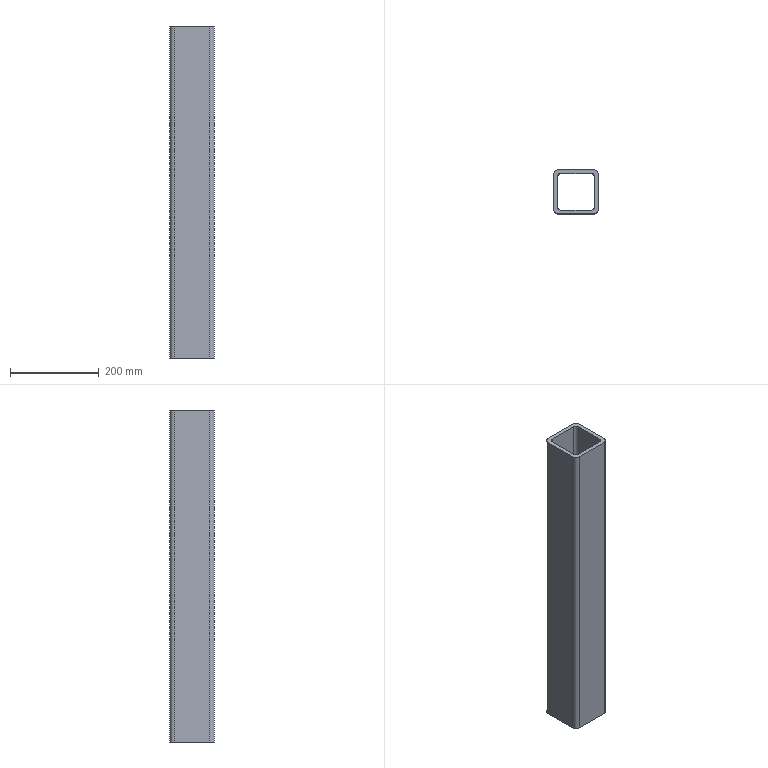Part | SolidWorks | features BaseBody 1 | 1 solid | 18 faces | box 100 x 100 x 750 mm | volume 2184823 mm3 | plane 10 | cylinder 8 | commonest cylinder face diameters 16 x4 20 x4
STEP:
#1=CARTESIAN_POINT('',(90.,-3.65,750.));
#2=VERTEX_POINT('',#1);
#3=CARTESIAN_POINT('',(90.,-3.65,0.));
#4=VERTEX_POINT('',#3);
#5=CARTESIAN_POINT('',(90.,-3.65,750.));
#6=DIRECTION('',(0.,0.,-1.));
#7=VECTOR('',#6,1000.);
#8=LINE('',#5,#7);
#9=EDGE_CURVE('',#2,#4,#8,.T.);
#10=ORIENTED_EDGE('',*,*,#9,.F.);
#11=CARTESIAN_POINT('',(10.,-3.65,750.));
#12=VERTEX_POINT('',#11);
#13=CARTESIAN_POINT('',(10.,-3.65,750.));
#14=DIRECTION('',(1.,0.,0.));
#15=VECTOR('',#14,1000.);
#16=LINE('',#13,#15);
#17=EDGE_CURVE('',#12,#2,#16,.T.);
#18=ORIENTED_EDGE('',*,*,#17,.F.);
#19=CARTESIAN_POINT('',(10.,-3.65,0.));
#20=VERTEX_POINT('',#19);
#21=CARTESIAN_POINT('',(10.,-3.65,750.));
#22=DIRECTION('',(0.,0.,1.));
#23=VECTOR('',#22,1000.);
#24=LINE('',#21,#23);
#25=EDGE_CURVE('',#20,#12,#24,.T.);
#26=ORIENTED_EDGE('',*,*,#25,.F.);
#27=CARTESIAN_POINT('',(10.,-3.65,0.));
#28=DIRECTION('',(-1.,0.,0.));
#29=VECTOR('',#28,1000.);
#30=LINE('',#27,#29);
#31=EDGE_CURVE('',#4,#20,#30,.T.);
#32=ORIENTED_EDGE('',*,*,#31,.F.);
#33=EDGE_LOOP('',(#10,#18,#26,#32));
#34=FACE_OUTER_BOUND('',#33,.T.);
#35=CARTESIAN_POINT('',(10.,-3.65,750.));
#36=DIRECTION('',(0.,1.,0.));
#37=DIRECTION('',(-1.,0.,0.));
#38=AXIS2_PLACEMENT_3D('',#35,#36,#37);
#39=PLANE('',#38);
#40=ADVANCED_FACE('',(#34),#39,.F.);
#41=CARTESIAN_POINT('',(84.,4.35,0.));
#42=VERTEX_POINT('',#41);
#43=CARTESIAN_POINT('',(16.,4.35,0.));
#44=VERTEX_POINT('',#43);
#45=CARTESIAN_POINT('',(10.,4.35,0.));
#46=DIRECTION('',(-1.,0.,0.));
#47=VECTOR('',#46,1000.);
#48=LINE('',#45,#47);
#49=EDGE_CURVE('',#42,#44,#48,.T.);
#50=ORIENTED_EDGE('',*,*,#49,.F.);
#51=CARTESIAN_POINT('',(92.,12.35,0.));
#52=VERTEX_POINT('',#51);
#53=CARTESIAN_POINT('',(84.,12.35,0.));
#54=DIRECTION('',(0.,0.,-1.));
#55=DIRECTION('',(-1.,0.,0.));
#56=AXIS2_PLACEMENT_3D('',#53,#54,#55);
#57=CIRCLE('',#56,8.);
#58=EDGE_CURVE('',#52,#42,#57,.T.);
#59=ORIENTED_EDGE('',*,*,#58,.F.);
#60=CARTESIAN_POINT('',(92.,80.35,0.));
#61=VERTEX_POINT('',#60);
#62=CARTESIAN_POINT('',(92.,6.35,0.));
#63=DIRECTION('',(0.,-1.,0.));
#64=VECTOR('',#63,1000.);
#65=LINE('',#62,#64);
#66=EDGE_CURVE('',#61,#52,#65,.T.);
#67=ORIENTED_EDGE('',*,*,#66,.F.);
#68=CARTESIAN_POINT('',(84.,88.35,0.));
#69=VERTEX_POINT('',#68);
#70=CARTESIAN_POINT('',(84.,80.35,0.));
#71=DIRECTION('',(0.,0.,-1.));
#72=DIRECTION('',(-1.,0.,0.));
#73=AXIS2_PLACEMENT_3D('',#70,#71,#72);
#74=CIRCLE('',#73,8.);
#75=EDGE_CURVE('',#69,#61,#74,.T.);
#76=ORIENTED_EDGE('',*,*,#75,.F.);
#77=CARTESIAN_POINT('',(16.,88.35,0.));
#78=VERTEX_POINT('',#77);
#79=CARTESIAN_POINT('',(10.,88.35,0.));
#80=DIRECTION('',(1.,0.,0.));
#81=VECTOR('',#80,1000.);
#82=LINE('',#79,#81);
#83=EDGE_CURVE('',#78,#69,#82,.T.);
#84=ORIENTED_EDGE('',*,*,#83,.F.);
#85=CARTESIAN_POINT('',(8.,80.35,0.));
#86=VERTEX_POINT('',#85);
#87=CARTESIAN_POINT('',(16.,80.35,0.));
#88=DIRECTION('',(0.,0.,-1.));
#89=DIRECTION('',(-1.,0.,0.));
#90=AXIS2_PLACEMENT_3D('',#87,#88,#89);
#91=CIRCLE('',#90,8.);
#92=EDGE_CURVE('',#86,#78,#91,.T.);
#93=ORIENTED_EDGE('',*,*,#92,.F.);
#94=CARTESIAN_POINT('',(8.,12.35,0.));
#95=VERTEX_POINT('',#94);
#96=CARTESIAN_POINT('',(8.,6.35,0.));
#97=DIRECTION('',(0.,1.,0.));
#98=VECTOR('',#97,1000.);
#99=LINE('',#96,#98);
#100=EDGE_CURVE('',#95,#86,#99,.T.);
#101=ORIENTED_EDGE('',*,*,#100,.F.);
#102=CARTESIAN_POINT('',(16.,12.35,0.));
#103=DIRECTION('',(0.,0.,-1.));
#104=DIRECTION('',(-1.,0.,0.));
#105=AXIS2_PLACEMENT_3D('',#102,#103,#104);
#106=CIRCLE('',#105,8.);
#107=EDGE_CURVE('',#44,#95,#106,.T.);
#108=ORIENTED_EDGE('',*,*,#107,.F.);
#109=EDGE_LOOP('',(#50,#59,#67,#76,#84,#93,#101,#108));
#110=FACE_BOUND('',#109,.T.);
#111=CARTESIAN_POINT('',(0.,86.35,0.));
#112=VERTEX_POINT('',#111);
#113=CARTESIAN_POINT('',(0.,6.35,0.));
#114=VERTEX_POINT('',#113);
#115=CARTESIAN_POINT('',(0.,6.35,0.));
#116=DIRECTION('',(0.,-1.,0.));
#117=VECTOR('',#116,1000.);
#118=LINE('',#115,#117);
#119=EDGE_CURVE('',#112,#114,#118,.T.);
#120=ORIENTED_EDGE('',*,*,#119,.F.);
#121=CARTESIAN_POINT('',(10.,96.35,0.));
#122=VERTEX_POINT('',#121);
#123=CARTESIAN_POINT('',(10.,86.35,0.));
#124=DIRECTION('',(0.,0.,1.));
#125=DIRECTION('',(-1.,0.,0.));
#126=AXIS2_PLACEMENT_3D('',#123,#124,#125);
#127=CIRCLE('',#126,10.);
#128=EDGE_CURVE('',#122,#112,#127,.T.);
#129=ORIENTED_EDGE('',*,*,#128,.F.);
#130=CARTESIAN_POINT('',(90.,96.35,0.));
#131=VERTEX_POINT('',#130);
#132=CARTESIAN_POINT('',(10.,96.35,0.));
#133=DIRECTION('',(-1.,0.,0.));
#134=VECTOR('',#133,1000.);
#135=LINE('',#132,#134);
#136=EDGE_CURVE('',#131,#122,#135,.T.);
#137=ORIENTED_EDGE('',*,*,#136,.F.);
#138=CARTESIAN_POINT('',(100.,86.35,0.));
#139=VERTEX_POINT('',#138);
#140=CARTESIAN_POINT('',(90.,86.35,0.));
#141=DIRECTION('',(0.,0.,1.));
#142=DIRECTION('',(-1.,0.,0.));
#143=AXIS2_PLACEMENT_3D('',#140,#141,#142);
#144=CIRCLE('',#143,10.);
#145=EDGE_CURVE('',#139,#131,#144,.T.);
#146=ORIENTED_EDGE('',*,*,#145,.F.);
#147=CARTESIAN_POINT('',(100.,6.35,0.));
#148=VERTEX_POINT('',#147);
#149=CARTESIAN_POINT('',(100.,6.35,0.));
#150=DIRECTION('',(0.,1.,0.));
#151=VECTOR('',#150,1000.);
#152=LINE('',#149,#151);
#153=EDGE_CURVE('',#148,#139,#152,.T.);
#154=ORIENTED_EDGE('',*,*,#153,.F.);
#155=CARTESIAN_POINT('',(90.,6.35,0.));
#156=DIRECTION('',(0.,0.,1.));
#157=DIRECTION('',(-1.,0.,0.));
#158=AXIS2_PLACEMENT_3D('',#155,#156,#157);
#159=CIRCLE('',#158,10.);
#160=EDGE_CURVE('',#4,#148,#159,.T.);
#161=ORIENTED_EDGE('',*,*,#160,.F.);
#162=ORIENTED_EDGE('',*,*,#31,.T.);
#163=CARTESIAN_POINT('',(10.,6.35,0.));
#164=DIRECTION('',(0.,0.,1.));
#165=DIRECTION('',(-1.,0.,0.));
#166=AXIS2_PLACEMENT_3D('',#163,#164,#165);
#167=CIRCLE('',#166,10.);
#168=EDGE_CURVE('',#114,#20,#167,.T.);
#169=ORIENTED_EDGE('',*,*,#168,.F.);
#170=EDGE_LOOP('',(#120,#129,#137,#146,#154,#161,#162,#169));
#171=FACE_OUTER_BOUND('',#170,.T.);
#172=CARTESIAN_POINT('',(10.,6.35,0.));
#173=DIRECTION('',(0.,0.,1.));
#174=DIRECTION('',(1.,0.,0.));
#175=AXIS2_PLACEMENT_3D('',#172,#173,#174);
#176=PLANE('',#175);
#177=ADVANCED_FACE('',(#110,#171),#176,.F.);
#178=CARTESIAN_POINT('',(100.,6.35,750.));
#179=VERTEX_POINT('',#178);
#180=CARTESIAN_POINT('',(90.,6.35,750.));
#181=DIRECTION('',(0.,0.,-1.));
#182=DIRECTION('',(-1.,0.,0.));
#183=AXIS2_PLACEMENT_3D('',#180,#181,#182);
#184=CIRCLE('',#183,10.);
#185=EDGE_CURVE('',#179,#2,#184,.T.);
#186=ORIENTED_EDGE('',*,*,#185,.T.);
#187=ORIENTED_EDGE('',*,*,#9,.T.);
#188=ORIENTED_EDGE('',*,*,#160,.T.);
#189=CARTESIAN_POINT('',(100.,6.35,750.));
#190=DIRECTION('',(0.,0.,1.));
#191=VECTOR('',#190,1000.);
#192=LINE('',#189,#191);
#193=EDGE_CURVE('',#148,#179,#192,.T.);
#194=ORIENTED_EDGE('',*,*,#193,.T.);
#195=EDGE_LOOP('',(#186,#187,#188,#194));
#196=FACE_OUTER_BOUND('',#195,.T.);
#197=CARTESIAN_POINT('',(90.,6.35,750.));
#198=DIRECTION('',(0.,0.,-1.));
#199=DIRECTION('',(-1.,0.,0.));
#200=AXIS2_PLACEMENT_3D('',#197,#198,#199);
#201=CYLINDRICAL_SURFACE('',#200,10.);
#202=ADVANCED_FACE('',(#196),#201,.T.);
#203=CARTESIAN_POINT('',(92.,80.35,750.));
#204=VERTEX_POINT('',#203);
#205=CARTESIAN_POINT('',(92.,12.35,750.));
#206=VERTEX_POINT('',#205);
#207=CARTESIAN_POINT('',(92.,6.35,750.));
#208=DIRECTION('',(0.,-1.,0.));
#209=VECTOR('',#208,1000.);
#210=LINE('',#207,#209);
#211=EDGE_CURVE('',#204,#206,#210,.T.);
#212=ORIENTED_EDGE('',*,*,#211,.T.);
#213=CARTESIAN_POINT('',(84.,4.35,750.));
#214=VERTEX_POINT('',#213);
#215=CARTESIAN_POINT('',(84.,12.35,750.));
#216=DIRECTION('',(0.,0.,-1.));
#217=DIRECTION('',(-1.,0.,0.));
#218=AXIS2_PLACEMENT_3D('',#215,#216,#217);
#219=CIRCLE('',#218,8.);
#220=EDGE_CURVE('',#206,#214,#219,.T.);
#221=ORIENTED_EDGE('',*,*,#220,.T.);
#222=CARTESIAN_POINT('',(16.,4.35,750.));
#223=VERTEX_POINT('',#222);
#224=CARTESIAN_POINT('',(10.,4.35,750.));
#225=DIRECTION('',(-1.,0.,0.));
#226=VECTOR('',#225,1000.);
#227=LINE('',#224,#226);
#228=EDGE_CURVE('',#214,#223,#227,.T.);
#229=ORIENTED_EDGE('',*,*,#228,.T.);
#230=CARTESIAN_POINT('',(8.,12.35,750.));
#231=VERTEX_POINT('',#230);
#232=CARTESIAN_POINT('',(16.,12.35,750.));
#233=DIRECTION('',(0.,0.,-1.));
#234=DIRECTION('',(-1.,0.,0.));
#235=AXIS2_PLACEMENT_3D('',#232,#233,#234);
#236=CIRCLE('',#235,8.);
#237=EDGE_CURVE('',#223,#231,#236,.T.);
#238=ORIENTED_EDGE('',*,*,#237,.T.);
#239=CARTESIAN_POINT('',(8.,80.35,750.));
#240=VERTEX_POINT('',#239);
#241=CARTESIAN_POINT('',(8.,6.35,750.));
#242=DIRECTION('',(0.,1.,0.));
#243=VECTOR('',#242,1000.);
#244=LINE('',#241,#243);
#245=EDGE_CURVE('',#231,#240,#244,.T.);
#246=ORIENTED_EDGE('',*,*,#245,.T.);
#247=CARTESIAN_POINT('',(16.,88.35,750.));
#248=VERTEX_POINT('',#247);
#249=CARTESIAN_POINT('',(16.,80.35,750.));
#250=DIRECTION('',(0.,0.,-1.));
#251=DIRECTION('',(-1.,0.,0.));
#252=AXIS2_PLACEMENT_3D('',#249,#250,#251);
#253=CIRCLE('',#252,8.);
#254=EDGE_CURVE('',#240,#248,#253,.T.);
#255=ORIENTED_EDGE('',*,*,#254,.T.);
#256=CARTESIAN_POINT('',(84.,88.35,750.));
#257=VERTEX_POINT('',#256);
#258=CARTESIAN_POINT('',(10.,88.35,750.));
#259=DIRECTION('',(1.,0.,0.));
#260=VECTOR('',#259,1000.);
#261=LINE('',#258,#260);
#262=EDGE_CURVE('',#248,#257,#261,.T.);
#263=ORIENTED_EDGE('',*,*,#262,.T.);
#264=CARTESIAN_POINT('',(84.,80.35,750.));
#265=DIRECTION('',(0.,0.,-1.));
#266=DIRECTION('',(-1.,0.,0.));
#267=AXIS2_PLACEMENT_3D('',#264,#265,#266);
#268=CIRCLE('',#267,8.);
#269=EDGE_CURVE('',#257,#204,#268,.T.);
#270=ORIENTED_EDGE('',*,*,#269,.T.);
#271=EDGE_LOOP('',(#212,#221,#229,#238,#246,#255,#263,#270));
#272=FACE_BOUND('',#271,.T.);
#273=CARTESIAN_POINT('',(10.,96.35,750.));
#274=VERTEX_POINT('',#273);
#275=CARTESIAN_POINT('',(0.,86.35,750.));
#276=VERTEX_POINT('',#275);
#277=CARTESIAN_POINT('',(10.,86.35,750.));
#278=DIRECTION('',(0.,0.,1.));
#279=DIRECTION('',(-1.,0.,0.));
#280=AXIS2_PLACEMENT_3D('',#277,#278,#279);
#281=CIRCLE('',#280,10.);
#282=EDGE_CURVE('',#274,#276,#281,.T.);
#283=ORIENTED_EDGE('',*,*,#282,.T.);
#284=CARTESIAN_POINT('',(0.,6.35,750.));
#285=VERTEX_POINT('',#284);
#286=CARTESIAN_POINT('',(0.,6.35,750.));
#287=DIRECTION('',(0.,-1.,0.));
#288=VECTOR('',#287,1000.);
#289=LINE('',#286,#288);
#290=EDGE_CURVE('',#276,#285,#289,.T.);
#291=ORIENTED_EDGE('',*,*,#290,.T.);
#292=CARTESIAN_POINT('',(10.,6.35,750.));
#293=DIRECTION('',(0.,0.,1.));
#294=DIRECTION('',(-1.,0.,0.));
#295=AXIS2_PLACEMENT_3D('',#292,#293,#294);
#296=CIRCLE('',#295,10.);
#297=EDGE_CURVE('',#285,#12,#296,.T.);
#298=ORIENTED_EDGE('',*,*,#297,.T.);
#299=ORIENTED_EDGE('',*,*,#17,.T.);
#300=ORIENTED_EDGE('',*,*,#185,.F.);
#301=CARTESIAN_POINT('',(100.,86.35,750.));
#302=VERTEX_POINT('',#301);
#303=CARTESIAN_POINT('',(100.,6.35,750.));
#304=DIRECTION('',(0.,1.,0.));
#305=VECTOR('',#304,1000.);
#306=LINE('',#303,#305);
#307=EDGE_CURVE('',#179,#302,#306,.T.);
#308=ORIENTED_EDGE('',*,*,#307,.T.);
#309=CARTESIAN_POINT('',(90.,96.35,750.));
#310=VERTEX_POINT('',#309);
#311=CARTESIAN_POINT('',(90.,86.35,750.));
#312=DIRECTION('',(0.,0.,1.));
#313=DIRECTION('',(-1.,0.,0.));
#314=AXIS2_PLACEMENT_3D('',#311,#312,#313);
#315=CIRCLE('',#314,10.);
#316=EDGE_CURVE('',#302,#310,#315,.T.);
#317=ORIENTED_EDGE('',*,*,#316,.T.);
#318=CARTESIAN_POINT('',(10.,96.35,750.));
#319=DIRECTION('',(-1.,0.,0.));
#320=VECTOR('',#319,1000.);
#321=LINE('',#318,#320);
#322=EDGE_CURVE('',#310,#274,#321,.T.);
#323=ORIENTED_EDGE('',*,*,#322,.T.);
#324=EDGE_LOOP('',(#283,#291,#298,#299,#300,#308,#317,#323));
#325=FACE_OUTER_BOUND('',#324,.T.);
#326=CARTESIAN_POINT('',(10.,6.35,750.));
#327=DIRECTION('',(0.,0.,1.));
#328=DIRECTION('',(1.,0.,0.));
#329=AXIS2_PLACEMENT_3D('',#326,#327,#328);
#330=PLANE('',#329);
#331=ADVANCED_FACE('',(#272,#325),#330,.T.);
#332=ORIENTED_EDGE('',*,*,#297,.F.);
#333=CARTESIAN_POINT('',(0.,6.35,750.));
#334=DIRECTION('',(0.,0.,-1.));
#335=VECTOR('',#334,1000.);
#336=LINE('',#333,#335);
#337=EDGE_CURVE('',#285,#114,#336,.T.);
#338=ORIENTED_EDGE('',*,*,#337,.T.);
#339=ORIENTED_EDGE('',*,*,#168,.T.);
#340=ORIENTED_EDGE('',*,*,#25,.T.);
#341=EDGE_LOOP('',(#332,#338,#339,#340));
#342=FACE_OUTER_BOUND('',#341,.T.);
#343=CARTESIAN_POINT('',(10.,6.35,750.));
#344=DIRECTION('',(0.,0.,-1.));
#345=DIRECTION('',(-1.,0.,0.));
#346=AXIS2_PLACEMENT_3D('',#343,#344,#345);
#347=CYLINDRICAL_SURFACE('',#346,10.);
#348=ADVANCED_FACE('',(#342),#347,.T.);
#349=CARTESIAN_POINT('',(8.,12.35,750.));
#350=DIRECTION('',(0.,0.,-1.));
#351=VECTOR('',#350,1000.);
#352=LINE('',#349,#351);
#353=EDGE_CURVE('',#231,#95,#352,.T.);
#354=ORIENTED_EDGE('',*,*,#353,.F.);
#355=ORIENTED_EDGE('',*,*,#237,.F.);
#356=CARTESIAN_POINT('',(16.,4.35,750.));
#357=DIRECTION('',(0.,0.,1.));
#358=VECTOR('',#357,1000.);
#359=LINE('',#356,#358);
#360=EDGE_CURVE('',#44,#223,#359,.T.);
#361=ORIENTED_EDGE('',*,*,#360,.F.);
#362=ORIENTED_EDGE('',*,*,#107,.T.);
#363=EDGE_LOOP('',(#354,#355,#361,#362));
#364=FACE_OUTER_BOUND('',#363,.T.);
#365=CARTESIAN_POINT('',(16.,12.35,750.));
#366=DIRECTION('',(0.,0.,-1.));
#367=DIRECTION('',(-1.,0.,0.));
#368=AXIS2_PLACEMENT_3D('',#365,#366,#367);
#369=CYLINDRICAL_SURFACE('',#368,8.);
#370=ADVANCED_FACE('',(#364),#369,.F.);
#371=ORIENTED_EDGE('',*,*,#228,.F.);
#372=CARTESIAN_POINT('',(84.,4.35,750.));
#373=DIRECTION('',(0.,0.,-1.));
#374=VECTOR('',#373,1000.);
#375=LINE('',#372,#374);
#376=EDGE_CURVE('',#214,#42,#375,.T.);
#377=ORIENTED_EDGE('',*,*,#376,.T.);
#378=ORIENTED_EDGE('',*,*,#49,.T.);
#379=ORIENTED_EDGE('',*,*,#360,.T.);
#380=EDGE_LOOP('',(#371,#377,#378,#379));
#381=FACE_OUTER_BOUND('',#380,.T.);
#382=CARTESIAN_POINT('',(16.,4.35,750.));
#383=DIRECTION('',(0.,1.,0.));
#384=DIRECTION('',(-1.,0.,0.));
#385=AXIS2_PLACEMENT_3D('',#382,#383,#384);
#386=PLANE('',#385);
#387=ADVANCED_FACE('',(#381),#386,.T.);
#388=ORIENTED_EDGE('',*,*,#376,.F.);
#389=ORIENTED_EDGE('',*,*,#220,.F.);
#390=CARTESIAN_POINT('',(92.,12.35,750.));
#391=DIRECTION('',(0.,0.,1.));
#392=VECTOR('',#391,1000.);
#393=LINE('',#390,#392);
#394=EDGE_CURVE('',#52,#206,#393,.T.);
#395=ORIENTED_EDGE('',*,*,#394,.F.);
#396=ORIENTED_EDGE('',*,*,#58,.T.);
#397=EDGE_LOOP('',(#388,#389,#395,#396));
#398=FACE_OUTER_BOUND('',#397,.T.);
#399=CARTESIAN_POINT('',(84.,12.35,750.));
#400=DIRECTION('',(0.,0.,-1.));
#401=DIRECTION('',(-1.,0.,0.));
#402=AXIS2_PLACEMENT_3D('',#399,#400,#401);
#403=CYLINDRICAL_SURFACE('',#402,8.);
#404=ADVANCED_FACE('',(#398),#403,.F.);
#405=ORIENTED_EDGE('',*,*,#394,.T.);
#406=ORIENTED_EDGE('',*,*,#211,.F.);
#407=CARTESIAN_POINT('',(92.,80.35,750.));
#408=DIRECTION('',(0.,0.,1.));
#409=VECTOR('',#408,1000.);
#410=LINE('',#407,#409);
#411=EDGE_CURVE('',#61,#204,#410,.T.);
#412=ORIENTED_EDGE('',*,*,#411,.F.);
#413=ORIENTED_EDGE('',*,*,#66,.T.);
#414=EDGE_LOOP('',(#405,#406,#412,#413));
#415=FACE_OUTER_BOUND('',#414,.T.);
#416=CARTESIAN_POINT('',(92.,80.35,750.));
#417=DIRECTION('',(1.,0.,0.));
#418=DIRECTION('',(0.,1.,0.));
#419=AXIS2_PLACEMENT_3D('',#416,#417,#418);
#420=PLANE('',#419);
#421=ADVANCED_FACE('',(#415),#420,.F.);
#422=ORIENTED_EDGE('',*,*,#411,.T.);
#423=ORIENTED_EDGE('',*,*,#269,.F.);
#424=CARTESIAN_POINT('',(84.,88.35,750.));
#425=DIRECTION('',(0.,0.,1.));
#426=VECTOR('',#425,1000.);
#427=LINE('',#424,#426);
#428=EDGE_CURVE('',#69,#257,#427,.T.);
#429=ORIENTED_EDGE('',*,*,#428,.F.);
#430=ORIENTED_EDGE('',*,*,#75,.T.);
#431=EDGE_LOOP('',(#422,#423,#429,#430));
#432=FACE_OUTER_BOUND('',#431,.T.);
#433=CARTESIAN_POINT('',(84.,80.35,750.));
#434=DIRECTION('',(0.,0.,-1.));
#435=DIRECTION('',(-1.,0.,0.));
#436=AXIS2_PLACEMENT_3D('',#433,#434,#435);
#437=CYLINDRICAL_SURFACE('',#436,8.);
#438=ADVANCED_FACE('',(#432),#437,.F.);
#439=ORIENTED_EDGE('',*,*,#262,.F.);
#440=CARTESIAN_POINT('',(16.,88.35,750.));
#441=DIRECTION('',(0.,0.,-1.));
#442=VECTOR('',#441,1000.);
#443=LINE('',#440,#442);
#444=EDGE_CURVE('',#248,#78,#443,.T.);
#445=ORIENTED_EDGE('',*,*,#444,.T.);
#446=ORIENTED_EDGE('',*,*,#83,.T.);
#447=ORIENTED_EDGE('',*,*,#428,.T.);
#448=EDGE_LOOP('',(#439,#445,#446,#447));
#449=FACE_OUTER_BOUND('',#448,.T.);
#450=CARTESIAN_POINT('',(84.,88.35,750.));
#451=DIRECTION('',(0.,-1.,0.));
#452=DIRECTION('',(1.,0.,0.));
#453=AXIS2_PLACEMENT_3D('',#450,#451,#452);
#454=PLANE('',#453);
#455=ADVANCED_FACE('',(#449),#454,.T.);
#456=ORIENTED_EDGE('',*,*,#444,.F.);
#457=ORIENTED_EDGE('',*,*,#254,.F.);
#458=CARTESIAN_POINT('',(8.,80.35,750.));
#459=DIRECTION('',(0.,0.,1.));
#460=VECTOR('',#459,1000.);
#461=LINE('',#458,#460);
#462=EDGE_CURVE('',#86,#240,#461,.T.);
#463=ORIENTED_EDGE('',*,*,#462,.F.);
#464=ORIENTED_EDGE('',*,*,#92,.T.);
#465=EDGE_LOOP('',(#456,#457,#463,#464));
#466=FACE_OUTER_BOUND('',#465,.T.);
#467=CARTESIAN_POINT('',(16.,80.35,750.));
#468=DIRECTION('',(0.,0.,-1.));
#469=DIRECTION('',(-1.,0.,0.));
#470=AXIS2_PLACEMENT_3D('',#467,#468,#469);
#471=CYLINDRICAL_SURFACE('',#470,8.);
#472=ADVANCED_FACE('',(#466),#471,.F.);
#473=ORIENTED_EDGE('',*,*,#462,.T.);
#474=ORIENTED_EDGE('',*,*,#245,.F.);
#475=ORIENTED_EDGE('',*,*,#353,.T.);
#476=ORIENTED_EDGE('',*,*,#100,.T.);
#477=EDGE_LOOP('',(#473,#474,#475,#476));
#478=FACE_OUTER_BOUND('',#477,.T.);
#479=CARTESIAN_POINT('',(8.,12.35,750.));
#480=DIRECTION('',(-1.,0.,0.));
#481=DIRECTION('',(0.,-1.,0.));
#482=AXIS2_PLACEMENT_3D('',#479,#480,#481);
#483=PLANE('',#482);
#484=ADVANCED_FACE('',(#478),#483,.F.);
#485=ORIENTED_EDGE('',*,*,#290,.F.);
#486=CARTESIAN_POINT('',(0.,86.35,750.));
#487=DIRECTION('',(0.,0.,-1.));
#488=VECTOR('',#487,1000.);
#489=LINE('',#486,#488);
#490=EDGE_CURVE('',#276,#112,#489,.T.);
#491=ORIENTED_EDGE('',*,*,#490,.T.);
#492=ORIENTED_EDGE('',*,*,#119,.T.);
#493=ORIENTED_EDGE('',*,*,#337,.F.);
#494=EDGE_LOOP('',(#485,#491,#492,#493));
#495=FACE_OUTER_BOUND('',#494,.T.);
#496=CARTESIAN_POINT('',(0.,6.35,750.));
#497=DIRECTION('',(-1.,0.,0.));
#498=DIRECTION('',(0.,-1.,0.));
#499=AXIS2_PLACEMENT_3D('',#496,#497,#498);
#500=PLANE('',#499);
#501=ADVANCED_FACE('',(#495),#500,.T.);
#502=ORIENTED_EDGE('',*,*,#282,.F.);
#503=CARTESIAN_POINT('',(10.,96.35,750.));
#504=DIRECTION('',(0.,0.,-1.));
#505=VECTOR('',#504,1000.);
#506=LINE('',#503,#505);
#507=EDGE_CURVE('',#274,#122,#506,.T.);
#508=ORIENTED_EDGE('',*,*,#507,.T.);
#509=ORIENTED_EDGE('',*,*,#128,.T.);
#510=ORIENTED_EDGE('',*,*,#490,.F.);
#511=EDGE_LOOP('',(#502,#508,#509,#510));
#512=FACE_OUTER_BOUND('',#511,.T.);
#513=CARTESIAN_POINT('',(10.,86.35,750.));
#514=DIRECTION('',(0.,0.,-1.));
#515=DIRECTION('',(-1.,0.,0.));
#516=AXIS2_PLACEMENT_3D('',#513,#514,#515);
#517=CYLINDRICAL_SURFACE('',#516,10.);
#518=ADVANCED_FACE('',(#512),#517,.T.);
#519=ORIENTED_EDGE('',*,*,#507,.F.);
#520=ORIENTED_EDGE('',*,*,#322,.F.);
#521=CARTESIAN_POINT('',(90.,96.35,750.));
#522=DIRECTION('',(0.,0.,1.));
#523=VECTOR('',#522,1000.);
#524=LINE('',#521,#523);
#525=EDGE_CURVE('',#131,#310,#524,.T.);
#526=ORIENTED_EDGE('',*,*,#525,.F.);
#527=ORIENTED_EDGE('',*,*,#136,.T.);
#528=EDGE_LOOP('',(#519,#520,#526,#527));
#529=FACE_OUTER_BOUND('',#528,.T.);
#530=CARTESIAN_POINT('',(90.,96.35,750.));
#531=DIRECTION('',(0.,-1.,0.));
#532=DIRECTION('',(1.,0.,0.));
#533=AXIS2_PLACEMENT_3D('',#530,#531,#532);
#534=PLANE('',#533);
#535=ADVANCED_FACE('',(#529),#534,.F.);
#536=ORIENTED_EDGE('',*,*,#316,.F.);
#537=CARTESIAN_POINT('',(100.,86.35,750.));
#538=DIRECTION('',(0.,0.,-1.));
#539=VECTOR('',#538,1000.);
#540=LINE('',#537,#539);
#541=EDGE_CURVE('',#302,#139,#540,.T.);
#542=ORIENTED_EDGE('',*,*,#541,.T.);
#543=ORIENTED_EDGE('',*,*,#145,.T.);
#544=ORIENTED_EDGE('',*,*,#525,.T.);
#545=EDGE_LOOP('',(#536,#542,#543,#544));
#546=FACE_OUTER_BOUND('',#545,.T.);
#547=CARTESIAN_POINT('',(90.,86.35,750.));
#548=DIRECTION('',(0.,0.,-1.));
#549=DIRECTION('',(-1.,0.,0.));
#550=AXIS2_PLACEMENT_3D('',#547,#548,#549);
#551=CYLINDRICAL_SURFACE('',#550,10.);
#552=ADVANCED_FACE('',(#546),#551,.T.);
#553=ORIENTED_EDGE('',*,*,#307,.F.);
#554=ORIENTED_EDGE('',*,*,#193,.F.);
#555=ORIENTED_EDGE('',*,*,#153,.T.);
#556=ORIENTED_EDGE('',*,*,#541,.F.);
#557=EDGE_LOOP('',(#553,#554,#555,#556));
#558=FACE_OUTER_BOUND('',#557,.T.);
#559=CARTESIAN_POINT('',(100.,86.35,750.));
#560=DIRECTION('',(1.,0.,0.));
#561=DIRECTION('',(0.,0.,-1.));
#562=AXIS2_PLACEMENT_3D('',#559,#560,#561);
#563=PLANE('',#562);
#564=ADVANCED_FACE('',(#558),#563,.T.);
#565=CLOSED_SHELL('',(#40,#177,#202,#331,#348,#370,#387,#404,#421,#438,#455,#472,#484,#501,#518,#535,#552,#564));
#566=MANIFOLD_SOLID_BREP('',#565);
#567=CARTESIAN_POINT('',(0.,0.,0.));
#568=DIRECTION('',(0.,0.,1.));
#569=DIRECTION('',(1.,0.,0.));
#570=AXIS2_PLACEMENT_3D('',#567,#568,#569);
#571=(LENGTH_UNIT()NAMED_UNIT(*)SI_UNIT(.MILLI.,.METRE.));
#572=UNCERTAINTY_MEASURE_WITH_UNIT(LENGTH_MEASURE(0.00001),#571,'','');
#573=(NAMED_UNIT(*)PLANE_ANGLE_UNIT()SI_UNIT($,.RADIAN.));
#574=(NAMED_UNIT(*)SI_UNIT($,.STERADIAN.)SOLID_ANGLE_UNIT());
#575=(GEOMETRIC_REPRESENTATION_CONTEXT(3)GLOBAL_UNCERTAINTY_ASSIGNED_CONTEXT((#572))GLOBAL_UNIT_ASSIGNED_CONTEXT((#571,#573,#574))REPRESENTATION_CONTEXT('',''));
#576=ADVANCED_BREP_SHAPE_REPRESENTATION('',(#566,#570),#575);